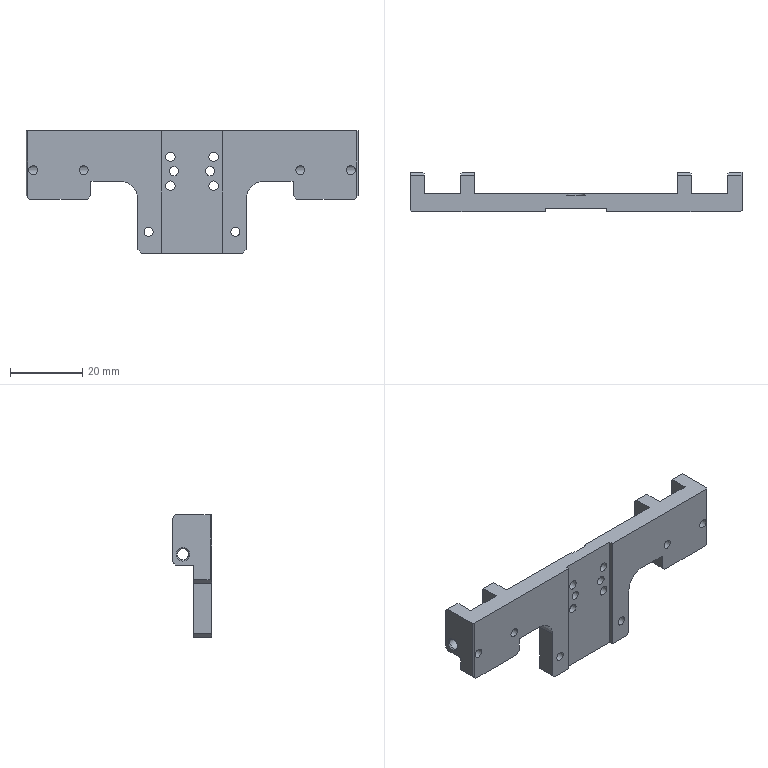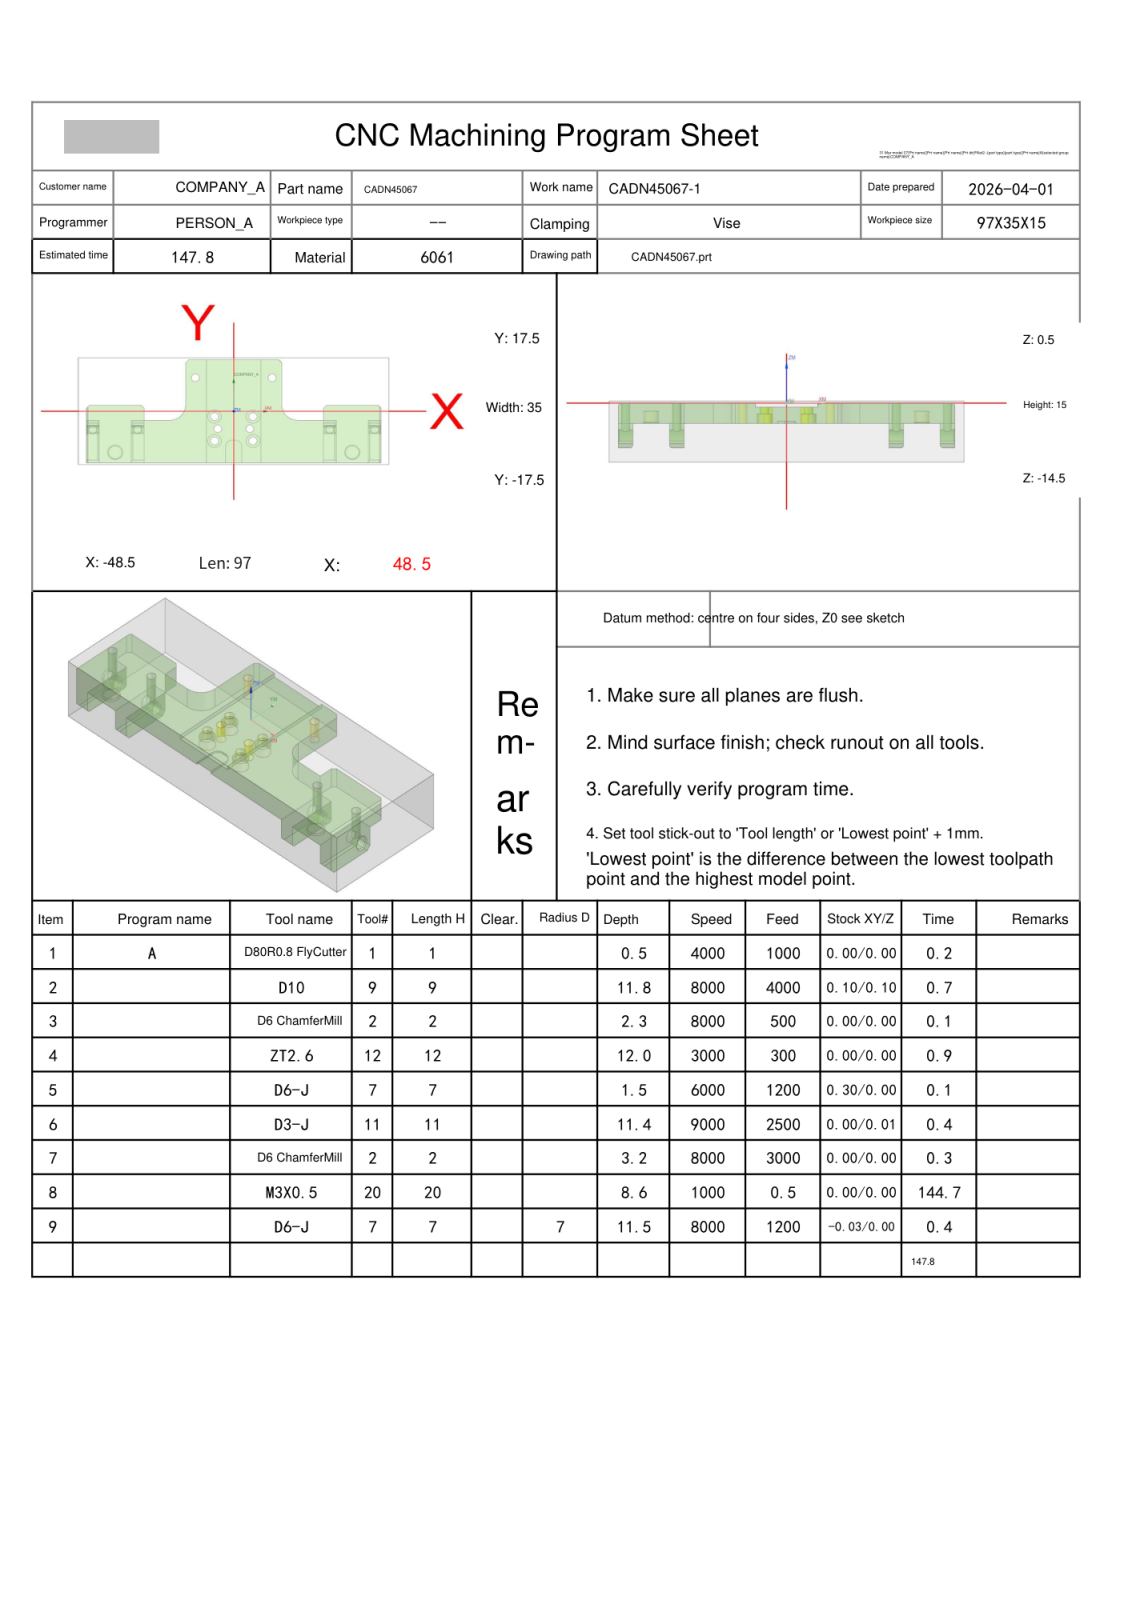NC program | NX | posted by the shop | part box 92 x 11 x 34 mm
Lines 974 to 3207 of 3207, first 1600 of 2234 lines:
N6 T11 M06
(D3-J  D=3. R=0. H=11 ce=0.00 di=0.01)
G00 G90 G54 X-26.294 Y2.051 M03 S9000
G43 H11 Z20.
M08
Z.154
G01 X-26.298 Y2.048 Z.09 F2000.
X-26.311 Y2.04 Z.031
X-26.332 Y2.027 Z-.021
X-26.357 Y2.009 Z-.068
X-26.388 Y1.987 Z-.11
X-26.421 Y1.961 Z-.147
X-26.456 Y1.932 Z-.178
X-26.491 Y1.9 Z-.206
X-26.525 Y1.865 Z-.229
X-26.556 Y1.828 Z-.248
X-26.584 Y1.79 Z-.264
X-26.607 Y1.75 Z-.276
X-26.623 Y1.708 Z-.285
X-26.631 Y1.667 Z-.291
X-26.63 Y1.625 Z-.295
X-26.618 Y1.583 Z-.296
G02 X-26.5 Y1. I-1.382 J-.583 F2500.
G01 Y-1.5
X-22.976
X-22.948 Y-1.485 Z-.297
X-22.944 Y-1.443 Z-.299
X-22.962 Y-1.377 Z-.304
X-23.001 Y-1.289 Z-.309
X-23.059 Y-1.182 Z-.316
X-23.134 Y-1.06 Z-.324
X-23.278 Y-.848 Z-.338
X-23.459 Y-.609 Z-.355
X-23.693 Y-.323 Z-.376
X-24. Y.01 Z-.403
X-24.329 Y.326 Z-.43
X-24.677 Y.621 Z-.458
X-25.039 Y.89 Z-.485
X-25.409 Y1.129 Z-.512
X-25.66 Y1.268 Z-.529
X-25.823 Y1.352 Z-.539
X-25.98 Y1.426 Z-.55
X-26.204 Y1.522 Z-.564
X-26.33 Y1.568 Z-.572
X-26.438 Y1.601 Z-.579
X-26.524 Y1.62 Z-.584
X-26.585 Y1.624 Z-.588
X-26.617 Y1.612 Z-.591
X-26.618 Y1.583 Z-.592
G02 X-26.5 Y1. I-1.382 J-.583
G01 Y-1.5
X-22.976
X-22.948 Y-1.485 Z-.593
X-22.944 Y-1.443 Z-.595
X-22.962 Y-1.377 Z-.6
X-23.001 Y-1.289 Z-.605
X-23.059 Y-1.182 Z-.612
X-23.134 Y-1.06 Z-.62
X-23.278 Y-.848 Z-.634
X-23.459 Y-.609 Z-.651
X-23.693 Y-.323 Z-.672
X-24. Y.01 Z-.699
X-24.329 Y.326 Z-.726
X-24.677 Y.621 Z-.754
X-25.039 Y.89 Z-.781
X-25.409 Y1.129 Z-.808
X-25.66 Y1.268 Z-.825
X-25.823 Y1.352 Z-.835
X-25.98 Y1.426 Z-.846
X-26.204 Y1.522 Z-.86
X-26.33 Y1.568 Z-.868
X-26.438 Y1.601 Z-.875
X-26.524 Y1.62 Z-.88
X-26.585 Y1.624 Z-.884
X-26.617 Y1.612 Z-.887
X-26.618 Y1.583 Z-.888
G02 X-26.5 Y1. I-1.382 J-.583
G01 Y-1.5
X-22.976
X-22.948 Y-1.485 Z-.889
X-22.944 Y-1.443 Z-.891
X-22.962 Y-1.377 Z-.895
X-23.001 Y-1.289 Z-.901
X-23.059 Y-1.182 Z-.908
X-23.134 Y-1.06 Z-.916
X-23.278 Y-.848 Z-.93
X-23.459 Y-.609 Z-.947
X-23.693 Y-.323 Z-.968
X-24. Y.01 Z-.995
X-24.329 Y.326 Z-1.022
X-24.677 Y.621 Z-1.05
X-25.039 Y.89 Z-1.077
X-25.409 Y1.129 Z-1.104
X-25.66 Y1.268 Z-1.121
X-25.823 Y1.352 Z-1.131
X-25.98 Y1.426 Z-1.141
X-26.204 Y1.522 Z-1.156
X-26.33 Y1.568 Z-1.164
X-26.438 Y1.601 Z-1.171
X-26.524 Y1.62 Z-1.176
X-26.585 Y1.624 Z-1.18
X-26.617 Y1.612 Z-1.183
X-26.618 Y1.583 Z-1.184
G02 X-26.5 Y1. I-1.382 J-.583
G01 Y-1.5
X-22.976
X-22.948 Y-1.485 Z-1.185
X-22.944 Y-1.443 Z-1.187
X-22.962 Y-1.377 Z-1.191
X-23.001 Y-1.289 Z-1.197
X-23.059 Y-1.182 Z-1.204
X-23.134 Y-1.06 Z-1.212
X-23.278 Y-.848 Z-1.226
X-23.459 Y-.609 Z-1.243
X-23.693 Y-.323 Z-1.264
X-24. Y.01 Z-1.29
X-24.329 Y.326 Z-1.318
X-24.677 Y.621 Z-1.346
X-25.039 Y.89 Z-1.373
X-25.409 Y1.129 Z-1.4
X-25.66 Y1.268 Z-1.417
X-25.823 Y1.352 Z-1.427
X-25.98 Y1.426 Z-1.437
X-26.204 Y1.522 Z-1.452
X-26.33 Y1.568 Z-1.46
X-26.438 Y1.601 Z-1.467
X-26.524 Y1.62 Z-1.472
X-26.585 Y1.624 Z-1.476
X-26.617 Y1.612 Z-1.479
X-26.618 Y1.583 Z-1.48
G02 X-26.5 Y1. I-1.382 J-.583
G01 Y-1.5
X-22.976
X-22.948 Y-1.485 Z-1.481
X-22.944 Y-1.443 Z-1.483
X-22.962 Y-1.377 Z-1.487
X-23.001 Y-1.289 Z-1.493
X-23.059 Y-1.182 Z-1.5
X-23.134 Y-1.06 Z-1.508
X-23.278 Y-.848 Z-1.522
X-23.459 Y-.609 Z-1.539
X-23.693 Y-.323 Z-1.56
X-24. Y.01 Z-1.586
X-24.329 Y.326 Z-1.614
X-24.677 Y.621 Z-1.642
X-25.039 Y.89 Z-1.669
X-25.409 Y1.129 Z-1.696
X-25.66 Y1.268 Z-1.712
X-25.823 Y1.352 Z-1.723
X-25.98 Y1.426 Z-1.733
X-26.204 Y1.522 Z-1.748
X-26.33 Y1.568 Z-1.756
X-26.438 Y1.601 Z-1.762
X-26.524 Y1.62 Z-1.768
X-26.585 Y1.624 Z-1.772
X-26.617 Y1.612 Z-1.775
X-26.618 Y1.583 Z-1.776
G02 X-26.5 Y1. I-1.382 J-.583
G01 Y-1.5
X-22.976
X-22.948 Y-1.485 Z-1.777
X-22.944 Y-1.443 Z-1.779
X-22.962 Y-1.377 Z-1.783
X-23.001 Y-1.289 Z-1.789
X-23.059 Y-1.182 Z-1.796
X-23.134 Y-1.06 Z-1.804
X-23.278 Y-.848 Z-1.818
X-23.459 Y-.609 Z-1.835
X-23.693 Y-.323 Z-1.856
X-24. Y.01 Z-1.882
X-24.329 Y.326 Z-1.91
X-24.677 Y.621 Z-1.938
X-25.039 Y.89 Z-1.965
X-25.409 Y1.129 Z-1.991
X-25.66 Y1.268 Z-2.008
X-25.823 Y1.352 Z-2.019
X-25.98 Y1.426 Z-2.029
X-26.204 Y1.522 Z-2.044
X-26.33 Y1.568 Z-2.052
X-26.438 Y1.601 Z-2.058
X-26.524 Y1.62 Z-2.064
X-26.585 Y1.624 Z-2.068
X-26.617 Y1.612 Z-2.071
X-26.618 Y1.583 Z-2.072
G02 X-26.5 Y1. I-1.382 J-.583
G01 Y-1.5
X-22.976
X-22.948 Y-1.485 Z-2.073
X-22.944 Y-1.443 Z-2.075
X-22.962 Y-1.377 Z-2.079
X-23.001 Y-1.289 Z-2.085
X-23.059 Y-1.182 Z-2.092
X-23.134 Y-1.06 Z-2.1
X-23.278 Y-.848 Z-2.114
X-23.459 Y-.609 Z-2.131
X-23.693 Y-.323 Z-2.152
X-24. Y.01 Z-2.178
X-24.329 Y.326 Z-2.206
X-24.677 Y.621 Z-2.233
X-25.039 Y.89 Z-2.261
X-25.409 Y1.129 Z-2.287
X-25.66 Y1.268 Z-2.304
X-25.823 Y1.352 Z-2.315
X-25.98 Y1.426 Z-2.325
X-26.204 Y1.522 Z-2.34
X-26.33 Y1.568 Z-2.348
X-26.438 Y1.601 Z-2.354
X-26.524 Y1.62 Z-2.36
X-26.585 Y1.624 Z-2.364
X-26.617 Y1.612 Z-2.367
X-26.618 Y1.583 Z-2.368
G02 X-26.5 Y1. I-1.382 J-.583
G01 Y-1.5
X-22.976
X-22.948 Y-1.485
X-22.944 Y-1.443 Z-2.371
X-22.962 Y-1.377 Z-2.375
X-23.001 Y-1.289 Z-2.381
X-23.059 Y-1.182 Z-2.388
X-23.134 Y-1.06 Z-2.396
X-23.278 Y-.848 Z-2.41
X-23.459 Y-.609 Z-2.427
X-23.693 Y-.323 Z-2.448
X-24. Y.01 Z-2.474
X-24.329 Y.326 Z-2.502
X-24.677 Y.621 Z-2.529
X-25.039 Y.89 Z-2.557
X-25.409 Y1.129 Z-2.583
X-25.66 Y1.268 Z-2.6
X-25.823 Y1.352 Z-2.611
X-25.98 Y1.426 Z-2.621
X-26.204 Y1.522 Z-2.635
X-26.33 Y1.568 Z-2.643
X-26.438 Y1.601 Z-2.65
X-26.524 Y1.62 Z-2.656
X-26.585 Y1.624 Z-2.66
X-26.617 Y1.612 Z-2.663
X-26.618 Y1.583 Z-2.664
G02 X-26.5 Y1. I-1.382 J-.583
G01 Y-1.5
X-22.976
X-22.948 Y-1.485
X-22.944 Y-1.443 Z-2.667
X-22.962 Y-1.377 Z-2.671
X-23.001 Y-1.289 Z-2.677
X-23.059 Y-1.182 Z-2.684
X-23.134 Y-1.06 Z-2.692
X-23.278 Y-.848 Z-2.706
X-23.459 Y-.609 Z-2.723
X-23.693 Y-.323 Z-2.744
X-24. Y.01 Z-2.77
X-24.329 Y.326 Z-2.798
X-24.677 Y.621 Z-2.825
X-25.039 Y.89 Z-2.853
X-25.409 Y1.129 Z-2.879
X-25.66 Y1.268 Z-2.896
X-25.823 Y1.352 Z-2.907
X-25.98 Y1.426 Z-2.917
X-26.204 Y1.522 Z-2.931
X-26.33 Y1.568 Z-2.939
X-26.438 Y1.601 Z-2.946
X-26.524 Y1.62 Z-2.952
X-26.585 Y1.624 Z-2.956
X-26.617 Y1.612 Z-2.959
X-26.618 Y1.583
G02 X-26.5 Y1. I-1.382 J-.583
G01 Y-1.5
X-22.976
X-22.948 Y-1.485 Z-2.96
X-22.944 Y-1.443 Z-2.963
X-22.962 Y-1.377 Z-2.967
X-23.001 Y-1.289 Z-2.973
X-23.059 Y-1.182 Z-2.979
X-23.134 Y-1.06 Z-2.987
X-23.278 Y-.848 Z-3.002
X-23.459 Y-.609 Z-3.019
X-23.693 Y-.323 Z-3.04
X-24. Y.01 Z-3.066
X-24.329 Y.326 Z-3.094
X-24.677 Y.621 Z-3.121
X-25.039 Y.89 Z-3.149
X-25.409 Y1.129 Z-3.175
X-25.66 Y1.268 Z-3.192
X-25.823 Y1.352 Z-3.203
X-25.98 Y1.426 Z-3.213
X-26.204 Y1.522 Z-3.227
X-26.33 Y1.568 Z-3.235
X-26.438 Y1.601 Z-3.242
X-26.524 Y1.62 Z-3.248
X-26.585 Y1.624 Z-3.252
X-26.617 Y1.612 Z-3.255
X-26.618 Y1.583
G02 X-26.5 Y1. I-1.382 J-.583
G01 Y-1.5
X-22.976
X-22.948 Y-1.485 Z-3.256
X-22.944 Y-1.443 Z-3.259
X-22.962 Y-1.377 Z-3.263
X-23.001 Y-1.289 Z-3.269
X-23.059 Y-1.182 Z-3.275
X-23.134 Y-1.06 Z-3.283
X-23.278 Y-.848 Z-3.298
X-23.459 Y-.609 Z-3.315
X-23.693 Y-.323 Z-3.336
X-24. Y.01 Z-3.362
X-24.329 Y.326 Z-3.39
X-24.677 Y.621 Z-3.417
X-25.039 Y.89 Z-3.445
X-25.409 Y1.129 Z-3.471
X-25.66 Y1.268 Z-3.488
X-25.823 Y1.352 Z-3.499
X-25.98 Y1.426 Z-3.509
X-26.204 Y1.522 Z-3.523
X-26.33 Y1.568 Z-3.531
X-26.438 Y1.601 Z-3.538
X-26.524 Y1.62 Z-3.544
X-26.585 Y1.624 Z-3.548
X-26.617 Y1.612 Z-3.55
X-26.618 Y1.583 Z-3.551
G02 X-26.5 Y1. I-1.382 J-.583
G01 Y-1.5
X-22.976
X-22.948 Y-1.485 Z-3.552
X-22.944 Y-1.443 Z-3.555
X-22.962 Y-1.377 Z-3.559
X-23.001 Y-1.289 Z-3.565
X-23.059 Y-1.182 Z-3.571
X-23.134 Y-1.06 Z-3.579
X-23.278 Y-.848 Z-3.594
X-23.459 Y-.609 Z-3.61
X-23.693 Y-.323 Z-3.632
X-24. Y.01 Z-3.658
X-24.329 Y.326 Z-3.685
X-24.677 Y.621 Z-3.713
X-25.039 Y.89 Z-3.741
X-25.409 Y1.129 Z-3.767
X-25.66 Y1.268 Z-3.784
X-25.823 Y1.352 Z-3.795
X-25.98 Y1.426 Z-3.805
X-26.204 Y1.522 Z-3.819
X-26.33 Y1.568 Z-3.827
X-26.438 Y1.601 Z-3.834
X-26.524 Y1.62 Z-3.84
X-26.585 Y1.624 Z-3.844
X-26.617 Y1.612 Z-3.846
X-26.618 Y1.583 Z-3.847
G02 X-26.5 Y1. I-1.382 J-.583
G01 Y-1.5
X-22.976
X-22.948 Y-1.485 Z-3.848
X-22.944 Y-1.443 Z-3.851
X-22.962 Y-1.377 Z-3.855
X-23.001 Y-1.289 Z-3.86
X-23.059 Y-1.182 Z-3.867
X-23.134 Y-1.06 Z-3.875
X-23.278 Y-.848 Z-3.89
X-23.459 Y-.609 Z-3.906
X-23.693 Y-.323 Z-3.927
X-24. Y.01 Z-3.954
X-24.329 Y.326 Z-3.981
X-24.677 Y.621 Z-4.009
X-25.039 Y.89 Z-4.037
X-25.409 Y1.129 Z-4.063
X-25.66 Y1.268 Z-4.08
X-25.823 Y1.352 Z-4.091
X-25.98 Y1.426 Z-4.101
X-26.204 Y1.522 Z-4.115
X-26.33 Y1.568 Z-4.123
X-26.438 Y1.601 Z-4.13
X-26.524 Y1.62 Z-4.136
X-26.585 Y1.624 Z-4.14
X-26.617 Y1.612 Z-4.142
X-26.618 Y1.583 Z-4.143
G02 X-26.5 Y1. I-1.382 J-.583
G01 Y-1.5
X-22.976
X-22.948 Y-1.485 Z-4.144
X-22.944 Y-1.443 Z-4.147
X-22.962 Y-1.377 Z-4.151
X-23.001 Y-1.289 Z-4.156
X-23.059 Y-1.182 Z-4.163
X-23.134 Y-1.06 Z-4.171
X-23.278 Y-.848 Z-4.186
X-23.459 Y-.609 Z-4.202
X-23.693 Y-.323 Z-4.223
X-24. Y.01 Z-4.25
X-24.329 Y.326 Z-4.277
X-24.677 Y.621 Z-4.305
X-25.039 Y.89 Z-4.333
X-25.409 Y1.129 Z-4.359
X-25.66 Y1.268 Z-4.376
X-25.823 Y1.352 Z-4.387
X-25.98 Y1.426 Z-4.397
X-26.204 Y1.522 Z-4.411
X-26.33 Y1.568 Z-4.419
X-26.438 Y1.601 Z-4.426
X-26.524 Y1.62 Z-4.432
X-26.585 Y1.624 Z-4.436
X-26.617 Y1.612 Z-4.438
X-26.618 Y1.583 Z-4.439
G02 X-26.5 Y1. I-1.382 J-.583
G01 Y-1.5
X-22.976
X-22.948 Y-1.485 Z-4.44
X-22.944 Y-1.443 Z-4.443
X-22.962 Y-1.377 Z-4.447
X-23.001 Y-1.289 Z-4.452
X-23.059 Y-1.182 Z-4.459
X-23.134 Y-1.06 Z-4.467
X-23.278 Y-.848 Z-4.481
X-23.459 Y-.609 Z-4.498
X-23.693 Y-.323 Z-4.519
X-24. Y.01 Z-4.546
X-24.329 Y.326 Z-4.573
X-24.677 Y.621 Z-4.601
X-25.039 Y.89 Z-4.628
X-25.409 Y1.129 Z-4.655
X-25.66 Y1.268 Z-4.672
X-25.823 Y1.352 Z-4.683
X-25.98 Y1.426 Z-4.693
X-26.204 Y1.522 Z-4.707
X-26.33 Y1.568 Z-4.715
X-26.438 Y1.601 Z-4.722
X-26.524 Y1.62 Z-4.728
X-26.585 Y1.624 Z-4.732
X-26.617 Y1.612 Z-4.734
X-26.618 Y1.583 Z-4.735
G02 X-26.5 Y1. I-1.382 J-.583
G01 Y-1.5
X-22.976
X-22.948 Y-1.485 Z-4.736
X-22.944 Y-1.443 Z-4.739
X-22.962 Y-1.377 Z-4.743
X-23.001 Y-1.289 Z-4.748
X-23.059 Y-1.182 Z-4.755
X-23.134 Y-1.06 Z-4.763
X-23.278 Y-.848 Z-4.777
X-23.459 Y-.609 Z-4.794
X-23.693 Y-.323 Z-4.815
X-24. Y.01 Z-4.842
X-24.33 Y.326 Z-4.869
X-24.677 Y.621 Z-4.897
X-25.039 Y.89 Z-4.924
X-25.41 Y1.129 Z-4.951
X-25.66 Y1.268 Z-4.968
X-25.823 Y1.352 Z-4.979
X-25.98 Y1.426 Z-4.989
X-26.204 Y1.522 Z-5.003
X-26.33 Y1.568 Z-5.011
X-26.438 Y1.601 Z-5.018
X-26.524 Y1.62 Z-5.023
X-26.585 Y1.624 Z-5.028
X-26.617 Y1.612 Z-5.03
X-26.618 Y1.583 Z-5.031
G02 X-26.5 Y1. I-1.382 J-.583
G01 Y-1.5
X-22.969
X-22.941 Y-1.485 Z-5.032
X-22.937 Y-1.443 Z-5.035
X-22.956 Y-1.377 Z-5.039
X-22.995 Y-1.289 Z-5.044
X-23.053 Y-1.182 Z-5.051
X-23.128 Y-1.06 Z-5.059
X-23.273 Y-.848 Z-5.073
X-23.454 Y-.609 Z-5.09
X-23.688 Y-.323 Z-5.111
X-23.996 Y.01 Z-5.138
X-24.326 Y.326 Z-5.165
X-24.674 Y.621 Z-5.193
X-25.036 Y.89 Z-5.22
X-25.408 Y1.129 Z-5.247
X-25.659 Y1.268 Z-5.264
X-25.822 Y1.352 Z-5.275
X-25.979 Y1.426 Z-5.285
X-26.204 Y1.522 Z-5.299
X-26.33 Y1.568 Z-5.307
X-26.438 Y1.601 Z-5.314
X-26.524 Y1.62 Z-5.319
X-26.585 Y1.624 Z-5.324
X-26.617 Y1.612 Z-5.326
X-26.618 Y1.583 Z-5.327
G02 X-26.5 Y1. I-1.382 J-.583
G01 Y-1.5
X-22.969
X-22.941 Y-1.485 Z-5.328
X-22.937 Y-1.443 Z-5.331
X-22.956 Y-1.377 Z-5.335
X-22.995 Y-1.289 Z-5.34
X-23.053 Y-1.182 Z-5.347
X-23.128 Y-1.06 Z-5.355
X-23.273 Y-.848 Z-5.369
X-23.454 Y-.609 Z-5.386
X-23.688 Y-.323 Z-5.407
X-23.996 Y.01 Z-5.434
X-24.326 Y.326 Z-5.461
X-24.674 Y.621 Z-5.489
X-25.036 Y.89 Z-5.516
X-25.408 Y1.129 Z-5.543
X-25.659 Y1.268 Z-5.56
X-25.822 Y1.352 Z-5.57
X-25.979 Y1.426 Z-5.581
X-26.204 Y1.522 Z-5.595
X-26.33 Y1.568 Z-5.603
X-26.438 Y1.601 Z-5.61
X-26.524 Y1.62 Z-5.615
X-26.585 Y1.624 Z-5.619
X-26.617 Y1.612 Z-5.622
X-26.618 Y1.583 Z-5.623
G02 X-26.5 Y1. I-1.382 J-.583
G01 Y-1.5
X-22.969
X-22.941 Y-1.485 Z-5.624
X-22.937 Y-1.443 Z-5.626
X-22.956 Y-1.377 Z-5.631
X-22.995 Y-1.289 Z-5.636
X-23.053 Y-1.182 Z-5.643
X-23.128 Y-1.06 Z-5.651
X-23.273 Y-.848 Z-5.665
X-23.454 Y-.609 Z-5.682
X-23.688 Y-.323 Z-5.703
X-23.996 Y.01 Z-5.73
X-24.326 Y.326 Z-5.757
X-24.674 Y.621 Z-5.785
X-25.036 Y.89 Z-5.812
X-25.408 Y1.129 Z-5.839
X-25.659 Y1.268 Z-5.856
X-25.822 Y1.352 Z-5.866
X-25.979 Y1.426 Z-5.877
X-26.204 Y1.522 Z-5.891
X-26.33 Y1.568 Z-5.899
X-26.438 Y1.601 Z-5.906
X-26.524 Y1.62 Z-5.911
X-26.585 Y1.624 Z-5.915
X-26.617 Y1.612 Z-5.918
X-26.618 Y1.583 Z-5.919
G02 X-26.5 Y1. I-1.382 J-.583
G01 Y-1.5
X-22.969
X-22.941 Y-1.485 Z-5.92
X-22.937 Y-1.443 Z-5.922
X-22.956 Y-1.377 Z-5.927
X-22.995 Y-1.289 Z-5.932
X-23.053 Y-1.182 Z-5.939
X-23.128 Y-1.06 Z-5.947
X-23.273 Y-.848 Z-5.961
X-23.454 Y-.609 Z-5.978
X-23.688 Y-.323 Z-5.999
X-23.996 Y.01 Z-6.026
X-24.326 Y.326 Z-6.053
X-24.674 Y.621 Z-6.081
X-25.036 Y.89 Z-6.108
X-25.408 Y1.129 Z-6.135
X-25.659 Y1.268 Z-6.152
X-25.822 Y1.352 Z-6.162
X-25.979 Y1.426 Z-6.172
X-26.204 Y1.522 Z-6.187
X-26.33 Y1.568 Z-6.195
X-26.438 Y1.601 Z-6.202
X-26.524 Y1.62 Z-6.207
X-26.585 Y1.624 Z-6.211
X-26.617 Y1.612 Z-6.214
X-26.618 Y1.583 Z-6.215
G02 X-26.5 Y1. I-1.382 J-.583
G01 Y-1.5
X-22.969
X-22.941 Y-1.485 Z-6.216
X-22.937 Y-1.443 Z-6.218
X-22.956 Y-1.377 Z-6.222
X-22.995 Y-1.289 Z-6.228
X-23.053 Y-1.182 Z-6.235
X-23.128 Y-1.06 Z-6.243
X-23.273 Y-.848 Z-6.257
X-23.454 Y-.609 Z-6.274
X-23.688 Y-.323 Z-6.295
X-23.996 Y.01 Z-6.322
X-24.326 Y.326 Z-6.349
X-24.674 Y.621 Z-6.377
X-25.036 Y.89 Z-6.404
X-25.408 Y1.129 Z-6.431
X-25.659 Y1.268 Z-6.448
X-25.822 Y1.352 Z-6.458
X-25.979 Y1.426 Z-6.468
X-26.204 Y1.522 Z-6.483
X-26.33 Y1.568 Z-6.491
X-26.438 Y1.601 Z-6.498
X-26.524 Y1.62 Z-6.503
X-26.585 Y1.624 Z-6.507
X-26.617 Y1.612 Z-6.51
X-26.618 Y1.583 Z-6.511
G02 X-26.5 Y1. I-1.382 J-.583
G01 Y-1.5
X-22.969
X-22.941 Y-1.485 Z-6.512
X-22.937 Y-1.443 Z-6.514
X-22.956 Y-1.377 Z-6.518
X-22.995 Y-1.289 Z-6.524
X-23.053 Y-1.182 Z-6.531
X-23.128 Y-1.06 Z-6.539
X-23.273 Y-.848 Z-6.553
X-23.454 Y-.609 Z-6.57
X-23.688 Y-.323 Z-6.591
X-23.996 Y.01 Z-6.617
X-24.326 Y.326 Z-6.645
X-24.674 Y.621 Z-6.673
X-25.036 Y.89 Z-6.7
X-25.408 Y1.129 Z-6.727
X-25.659 Y1.268 Z-6.744
X-25.822 Y1.352 Z-6.754
X-25.979 Y1.426 Z-6.764
X-26.204 Y1.522 Z-6.779
X-26.33 Y1.568 Z-6.787
X-26.438 Y1.601 Z-6.794
X-26.524 Y1.62 Z-6.799
X-26.585 Y1.624 Z-6.803
X-26.617 Y1.612 Z-6.806
X-26.618 Y1.583 Z-6.807
G02 X-26.5 Y1. I-1.382 J-.583
G01 Y-1.5
X-22.969
X-22.941 Y-1.485 Z-6.808
X-22.937 Y-1.443 Z-6.81
X-22.956 Y-1.377 Z-6.814
X-22.995 Y-1.289 Z-6.82
X-23.053 Y-1.182 Z-6.827
X-23.128 Y-1.06 Z-6.835
X-23.273 Y-.848 Z-6.849
X-23.454 Y-.609 Z-6.866
X-23.688 Y-.323 Z-6.887
X-23.996 Y.01 Z-6.913
X-24.326 Y.326 Z-6.941
X-24.674 Y.621 Z-6.969
X-25.036 Y.89 Z-6.996
X-25.408 Y1.129 Z-7.022
X-25.659 Y1.268 Z-7.039
X-25.822 Y1.352 Z-7.05
X-25.979 Y1.426 Z-7.06
X-26.204 Y1.522 Z-7.075
X-26.33 Y1.568 Z-7.083
X-26.438 Y1.601 Z-7.089
X-26.524 Y1.62 Z-7.095
X-26.585 Y1.624 Z-7.099
X-26.617 Y1.612 Z-7.102
X-26.618 Y1.583 Z-7.103
G02 X-26.5 Y1. I-1.382 J-.583
G01 Y-1.5
X-22.969
X-22.941 Y-1.485 Z-7.104
X-22.937 Y-1.443 Z-7.106
X-22.956 Y-1.377 Z-7.11
X-22.995 Y-1.289 Z-7.116
X-23.053 Y-1.182 Z-7.123
X-23.128 Y-1.06 Z-7.131
X-23.273 Y-.848 Z-7.145
X-23.454 Y-.609 Z-7.162
X-23.688 Y-.323 Z-7.183
X-23.996 Y.01 Z-7.209
X-24.326 Y.326 Z-7.237
X-24.674 Y.621 Z-7.264
X-25.036 Y.89 Z-7.292
X-25.408 Y1.129 Z-7.318
X-25.659 Y1.268 Z-7.335
X-25.822 Y1.352 Z-7.346
X-25.979 Y1.426 Z-7.356
X-26.204 Y1.522 Z-7.371
X-26.33 Y1.568 Z-7.379
X-26.438 Y1.601 Z-7.385
X-26.524 Y1.62 Z-7.391
X-26.585 Y1.624 Z-7.395
X-26.617 Y1.612 Z-7.398
X-26.618 Y1.583 Z-7.399
G02 X-26.5 Y1. I-1.382 J-.583
G01 Y-1.5
X-22.969
X-22.941 Y-1.485 Z-7.4
X-22.937 Y-1.443 Z-7.402
X-22.956 Y-1.377 Z-7.406
X-22.995 Y-1.289 Z-7.412
X-23.053 Y-1.182 Z-7.419
X-23.128 Y-1.06 Z-7.427
X-23.273 Y-.848 Z-7.441
X-23.454 Y-.609 Z-7.458
X-23.688 Y-.323 Z-7.479
X-23.996 Y.01 Z-7.505
X-24.326 Y.326 Z-7.533
X-24.674 Y.621 Z-7.56
X-25.036 Y.89 Z-7.588
X-25.408 Y1.129 Z-7.614
X-25.659 Y1.268 Z-7.631
X-25.822 Y1.352 Z-7.642
X-25.979 Y1.426 Z-7.652
X-26.204 Y1.522 Z-7.667
X-26.33 Y1.568 Z-7.675
X-26.438 Y1.601 Z-7.681
X-26.524 Y1.62 Z-7.687
X-26.585 Y1.624 Z-7.691
X-26.617 Y1.612 Z-7.694
X-26.618 Y1.583 Z-7.695
G02 X-26.5 Y1. I-1.382 J-.583
G01 Y-1.5
X-22.969
X-22.941 Y-1.485
X-22.937 Y-1.443 Z-7.698
X-22.956 Y-1.377 Z-7.702
X-22.995 Y-1.289 Z-7.708
X-23.053 Y-1.182 Z-7.715
X-23.128 Y-1.06 Z-7.723
X-23.273 Y-.848 Z-7.737
X-23.454 Y-.609 Z-7.754
X-23.688 Y-.323 Z-7.775
X-23.996 Y.01 Z-7.801
X-24.326 Y.326 Z-7.829
X-24.674 Y.621 Z-7.856
X-25.036 Y.89 Z-7.884
X-25.408 Y1.129 Z-7.91
X-25.659 Y1.268 Z-7.927
X-25.822 Y1.352 Z-7.938
X-25.979 Y1.426 Z-7.948
X-26.204 Y1.522 Z-7.962
X-26.33 Y1.568 Z-7.97
X-26.438 Y1.601 Z-7.977
X-26.524 Y1.62 Z-7.983
X-26.585 Y1.624 Z-7.987
X-26.617 Y1.612 Z-7.99
X-26.618 Y1.583 Z-7.991
G02 X-26.5 Y1. I-1.382 J-.583
G01 Y-1.5
X-22.969
X-22.941 Y-1.485
X-22.937 Y-1.443 Z-7.994
X-22.956 Y-1.377 Z-7.998
X-22.995 Y-1.289 Z-8.004
X-23.053 Y-1.182 Z-8.011
X-23.128 Y-1.06 Z-8.019
X-23.273 Y-.848 Z-8.033
X-23.454 Y-.609 Z-8.05
X-23.688 Y-.323 Z-8.071
X-23.996 Y.01 Z-8.097
X-24.326 Y.326 Z-8.125
X-24.674 Y.621 Z-8.152
X-25.036 Y.89 Z-8.18
X-25.408 Y1.129 Z-8.206
X-25.659 Y1.268 Z-8.223
X-25.822 Y1.352 Z-8.234
X-25.979 Y1.426 Z-8.244
X-26.204 Y1.522 Z-8.258
X-26.33 Y1.568 Z-8.266
X-26.438 Y1.601 Z-8.273
X-26.524 Y1.62 Z-8.279
X-26.585 Y1.624 Z-8.283
X-26.617 Y1.612 Z-8.286
X-26.618 Y1.583
G02 X-26.5 Y1. I-1.382 J-.583
G01 Y-1.5
X-22.969
X-22.941 Y-1.485 Z-8.287
X-22.937 Y-1.443 Z-8.29
X-22.956 Y-1.377 Z-8.294
X-22.995 Y-1.289 Z-8.3
X-23.053 Y-1.182 Z-8.307
X-23.128 Y-1.06 Z-8.314
X-23.273 Y-.848 Z-8.329
X-23.454 Y-.609 Z-8.346
X-23.688 Y-.323 Z-8.367
X-23.996 Y.01 Z-8.393
X-24.326 Y.326 Z-8.421
X-24.674 Y.621 Z-8.448
X-25.036 Y.89 Z-8.476
X-25.408 Y1.129 Z-8.502
X-25.659 Y1.268 Z-8.519
X-25.822 Y1.352 Z-8.53
X-25.979 Y1.426 Z-8.54
X-26.204 Y1.522 Z-8.554
X-26.33 Y1.568 Z-8.562
X-26.438 Y1.601 Z-8.569
X-26.524 Y1.62 Z-8.575
X-26.585 Y1.624 Z-8.579
X-26.617 Y1.612 Z-8.582
X-26.618 Y1.583
G02 X-26.5 Y1. I-1.382 J-.583
G01 Y-1.5
X-22.969
X-22.941 Y-1.485 Z-8.583
X-22.937 Y-1.443 Z-8.586
X-22.956 Y-1.377 Z-8.59
X-22.995 Y-1.289 Z-8.596
X-23.053 Y-1.182 Z-8.602
X-23.128 Y-1.06 Z-8.61
X-23.273 Y-.848 Z-8.625
X-23.454 Y-.609 Z-8.642
X-23.688 Y-.323 Z-8.663
X-23.996 Y.01 Z-8.689
X-24.326 Y.326 Z-8.716
X-24.674 Y.621 Z-8.744
X-25.036 Y.89 Z-8.772
X-25.408 Y1.129 Z-8.798
X-25.659 Y1.269 Z-8.815
X-25.822 Y1.352 Z-8.826
X-25.979 Y1.426 Z-8.836
X-26.204 Y1.522 Z-8.85
X-26.33 Y1.568 Z-8.858
X-26.438 Y1.601 Z-8.865
X-26.524 Y1.62 Z-8.871
X-26.585 Y1.624 Z-8.875
X-26.617 Y1.612 Z-8.877
X-26.618 Y1.583 Z-8.878
G02 X-26.5 Y1. I-1.382 J-.583
G01 Y-1.5
X-22.969
X-22.941 Y-1.485 Z-8.879
X-22.937 Y-1.443 Z-8.882
X-22.956 Y-1.377 Z-8.886
X-22.995 Y-1.289 Z-8.892
X-23.053 Y-1.182 Z-8.898
X-23.128 Y-1.06 Z-8.906
X-23.273 Y-.848 Z-8.921
X-23.454 Y-.609 Z-8.937
X-23.688 Y-.323 Z-8.958
X-23.996 Y.01 Z-8.985
X-24.326 Y.326 Z-9.012
X-24.674 Y.621 Z-9.04
X-25.036 Y.89 Z-9.068
X-25.408 Y1.129 Z-9.094
X-25.659 Y1.269 Z-9.111
X-25.822 Y1.352 Z-9.122
X-25.979 Y1.426 Z-9.132
X-26.204 Y1.522 Z-9.146
X-26.33 Y1.568 Z-9.154
X-26.438 Y1.601 Z-9.161
X-26.524 Y1.62 Z-9.167
X-26.585 Y1.624 Z-9.171
X-26.617 Y1.612 Z-9.173
X-26.618 Y1.583 Z-9.174
G02 X-26.5 Y1. I-1.382 J-.583
G01 Y-1.5
X-22.969
X-22.941 Y-1.485 Z-9.175
X-22.937 Y-1.443 Z-9.178
X-22.956 Y-1.377 Z-9.182
X-22.995 Y-1.289 Z-9.188
X-23.053 Y-1.182 Z-9.194
X-23.128 Y-1.06 Z-9.202
X-23.273 Y-.848 Z-9.217
X-23.454 Y-.609 Z-9.233
X-23.688 Y-.323 Z-9.254
X-23.996 Y.01 Z-9.281
X-24.326 Y.326 Z-9.308
X-24.674 Y.621 Z-9.336
X-25.036 Y.89 Z-9.364
X-25.408 Y1.129 Z-9.39
X-25.659 Y1.269 Z-9.407
X-25.822 Y1.352 Z-9.418
X-25.979 Y1.426 Z-9.428
X-26.204 Y1.522 Z-9.442
X-26.33 Y1.568 Z-9.45
X-26.438 Y1.601 Z-9.457
X-26.524 Y1.62 Z-9.463
X-26.585 Y1.624 Z-9.467
X-26.617 Y1.612 Z-9.469
X-26.618 Y1.583 Z-9.47
G02 X-26.5 Y1. I-1.382 J-.583
G01 Y-1.5
X-22.969
X-22.941 Y-1.485 Z-9.471
X-22.937 Y-1.443 Z-9.474
X-22.956 Y-1.377 Z-9.478
X-22.995 Y-1.289 Z-9.483
X-23.053 Y-1.182 Z-9.49
X-23.128 Y-1.06 Z-9.498
X-23.273 Y-.848 Z-9.513
X-23.454 Y-.609 Z-9.529
X-23.688 Y-.323 Z-9.55
X-23.996 Y.01 Z-9.577
X-24.326 Y.326 Z-9.604
X-24.674 Y.621 Z-9.632
X-25.036 Y.89 Z-9.659
X-25.408 Y1.129 Z-9.686
X-25.659 Y1.269 Z-9.703
X-25.822 Y1.352 Z-9.714
X-25.979 Y1.426 Z-9.724
X-26.204 Y1.522 Z-9.738
X-26.33 Y1.568 Z-9.746
X-26.438 Y1.601 Z-9.753
X-26.524 Y1.62 Z-9.759
X-26.585 Y1.624 Z-9.763
X-26.617 Y1.612 Z-9.765
X-26.618 Y1.583 Z-9.766
G02 X-26.5 Y1. I-1.382 J-.583
G01 Y-1.5
X-22.969
X-22.941 Y-1.485 Z-9.767
X-22.937 Y-1.443 Z-9.77
X-22.956 Y-1.377 Z-9.774
X-22.995 Y-1.289 Z-9.779
X-23.053 Y-1.182 Z-9.786
X-23.128 Y-1.06 Z-9.794
X-23.273 Y-.848 Z-9.809
X-23.454 Y-.609 Z-9.825
X-23.688 Y-.323 Z-9.846
X-23.996 Y.01 Z-9.873
X-24.326 Y.326 Z-9.9
X-24.674 Y.621 Z-9.928
X-25.036 Y.89 Z-9.955
X-25.408 Y1.129 Z-9.982
X-25.659 Y1.269 Z-9.999
X-25.822 Y1.352 Z-10.01
X-25.979 Y1.426 Z-10.02
X-26.204 Y1.522 Z-10.034
X-26.33 Y1.568 Z-10.042
X-26.438 Y1.601 Z-10.049
X-26.524 Y1.62 Z-10.055
X-26.585 Y1.624 Z-10.059
X-26.617 Y1.612 Z-10.061
X-26.618 Y1.583 Z-10.062
G02 X-26.5 Y1. I-1.382 J-.583
G01 Y-1.5
X-22.969
X-22.941 Y-1.485 Z-10.063
X-22.937 Y-1.443 Z-10.066
X-22.956 Y-1.377 Z-10.07
X-22.995 Y-1.289 Z-10.075
X-23.053 Y-1.182 Z-10.082
X-23.128 Y-1.06 Z-10.09
X-23.273 Y-.848 Z-10.104
X-23.454 Y-.609 Z-10.121
X-23.688 Y-.323 Z-10.142
X-23.996 Y.01 Z-10.169
X-24.326 Y.326 Z-10.196
X-24.674 Y.621 Z-10.224
X-25.036 Y.89 Z-10.251
X-25.408 Y1.129 Z-10.278
X-25.659 Y1.269 Z-10.295
X-25.822 Y1.352 Z-10.306
X-25.979 Y1.426 Z-10.316
X-26.204 Y1.522 Z-10.33
X-26.33 Y1.568 Z-10.338
X-26.438 Y1.601 Z-10.345
X-26.524 Y1.62 Z-10.35
X-26.585 Y1.624 Z-10.355
X-26.617 Y1.612 Z-10.357
X-26.618 Y1.583 Z-10.358
G02 X-26.5 Y1. I-1.382 J-.583
G01 Y-1.5
X-22.969
X-22.941 Y-1.485 Z-10.359
X-22.937 Y-1.443 Z-10.362
X-22.956 Y-1.377 Z-10.366
X-22.995 Y-1.289 Z-10.371
X-23.053 Y-1.182 Z-10.378
X-23.128 Y-1.06 Z-10.386
X-23.273 Y-.848 Z-10.4
X-23.454 Y-.609 Z-10.417
X-23.688 Y-.323 Z-10.438
X-23.996 Y.01 Z-10.465
X-24.326 Y.326 Z-10.492
X-24.674 Y.621 Z-10.52
X-25.036 Y.89 Z-10.547
X-25.408 Y1.129 Z-10.574
X-25.659 Y1.269 Z-10.591
X-25.822 Y1.352 Z-10.602
X-25.979 Y1.426 Z-10.612
X-26.204 Y1.522 Z-10.626
X-26.33 Y1.568 Z-10.634
X-26.438 Y1.601 Z-10.641
X-26.524 Y1.62 Z-10.646
X-26.585 Y1.624 Z-10.651
X-26.617 Y1.612 Z-10.653
X-26.618 Y1.583 Z-10.654
G02 X-26.5 Y1. I-1.382 J-.583
G01 Y-1.5
X-22.969
X-22.941 Y-1.485 Z-10.655
X-22.937 Y-1.443 Z-10.658
X-22.956 Y-1.377 Z-10.662
X-22.995 Y-1.289 Z-10.667
X-23.053 Y-1.182 Z-10.674
X-23.128 Y-1.06 Z-10.682
X-23.273 Y-.848 Z-10.696
X-23.454 Y-.609 Z-10.713
X-23.688 Y-.323 Z-10.734
X-23.996 Y.01 Z-10.761
X-24.326 Y.326 Z-10.788
X-24.674 Y.621 Z-10.816
X-25.036 Y.89 Z-10.843
X-25.408 Y1.129 Z-10.87
X-25.659 Y1.269 Z-10.887
X-25.822 Y1.352 Z-10.898
X-25.979 Y1.426 Z-10.908
X-26.204 Y1.522 Z-10.922
X-26.33 Y1.568 Z-10.93
X-26.438 Y1.601 Z-10.937
X-26.524 Y1.62 Z-10.942
X-26.585 Y1.624 Z-10.947
X-26.617 Y1.612 Z-10.949
X-26.618 Y1.583 Z-10.95
G02 X-26.5 Y1. I-1.382 J-.583
G01 Y-1.5
X-22.969
X-22.928 Y-1.475 Z-10.949
X-22.891 Y-1.441 Z-10.945
X-22.858 Y-1.401 Z-10.938
X-22.828 Y-1.355 Z-10.927
X-22.802 Y-1.305 Z-10.913
X-22.78 Y-1.253 Z-10.895
X-22.76 Y-1.2 Z-10.873
X-22.744 Y-1.147 Z-10.846
X-22.731 Y-1.097 Z-10.814
X-22.72 Y-1.05 Z-10.777
X-22.711 Y-1.009 Z-10.734
X-22.705 Y-.973 Z-10.685
X-22.701 Y-.947 Z-10.63
X-22.698 Y-.929 Z-10.568
X-22.697 Y-.923 Z-10.5
G00 Z20.
X22.725 Y-.914
Z.154
G01 X22.726 Y-.92 Z.086 F2000.
X22.727 Y-.938 Z.024
X22.73 Y-.965 Z-.031
X22.735 Y-1.001 Z-.08
X22.742 Y-1.043 Z-.123
X22.751 Y-1.091 Z-.16
X22.762 Y-1.142 Z-.192
X22.776 Y-1.196 Z-.219
X22.794 Y-1.25 Z-.241
X22.814 Y-1.303 Z-.259
X22.838 Y-1.354 Z-.273
X22.866 Y-1.4 Z-.284
X22.898 Y-1.441 Z-.291
X22.935 Y-1.475 Z-.295
X22.976 Y-1.5 Z-.296
X26.5 F2500.
Y1.
G02 X26.618 Y1.583 I1.5 J0.0
G01 X26.617 Y1.612 Z-.297
X26.586 Y1.624 Z-.299
X26.526 Y1.619 Z-.304
X26.442 Y1.6 Z-.309
X26.336 Y1.566 Z-.316
X26.212 Y1.519 Z-.324
X25.991 Y1.422 Z-.338
X25.736 Y1.295 Z-.355
X25.428 Y1.123 Z-.376
X25.06 Y.885 Z-.403
X24.7 Y.617 Z-.43
X24.352 Y.323 Z-.458
X24.02 Y.008 Z-.485
X23.711 Y-.323 Z-.512
X23.473 Y-.608 Z-.533
X23.336 Y-.786 Z-.545
X23.141 Y-1.06 Z-.564
X23.065 Y-1.182 Z-.572
X23.005 Y-1.288 Z-.579
X22.964 Y-1.376 Z-.584
X22.945 Y-1.443 Z-.588
X22.948 Y-1.485 Z-.591
X22.976 Y-1.5 Z-.592
X26.5
Y1.
G02 X26.618 Y1.583 I1.5 J0.0
G01 X26.617 Y1.612 Z-.593
X26.586 Y1.624 Z-.595
X26.526 Y1.619 Z-.6
X26.442 Y1.6 Z-.605
X26.336 Y1.566 Z-.612
X26.212 Y1.519 Z-.62
X25.991 Y1.422 Z-.634
X25.736 Y1.295 Z-.651
X25.428 Y1.123 Z-.672
X25.06 Y.885 Z-.699
X24.7 Y.617 Z-.726
X24.352 Y.323 Z-.754
X24.02 Y.008 Z-.781
X23.711 Y-.323 Z-.808
X23.473 Y-.608 Z-.829
X23.336 Y-.786 Z-.841
X23.141 Y-1.06 Z-.86
X23.065 Y-1.182 Z-.868
X23.005 Y-1.288 Z-.875
X22.964 Y-1.376 Z-.88
X22.945 Y-1.443 Z-.884
X22.948 Y-1.485 Z-.887
X22.976 Y-1.5 Z-.888
X26.5
Y1.
G02 X26.618 Y1.583 I1.5 J0.0
G01 X26.617 Y1.612 Z-.889
X26.586 Y1.624 Z-.891
X26.526 Y1.619 Z-.895
X26.442 Y1.6 Z-.901
X26.336 Y1.566 Z-.908
X26.212 Y1.519 Z-.916
X25.991 Y1.422 Z-.93
X25.736 Y1.295 Z-.947
X25.428 Y1.123 Z-.968
X25.06 Y.885 Z-.995
X24.7 Y.617 Z-1.022
X24.352 Y.323 Z-1.05
X24.02 Y.008 Z-1.077
X23.711 Y-.323 Z-1.104
X23.473 Y-.608 Z-1.125
X23.336 Y-.786 Z-1.137
X23.141 Y-1.06 Z-1.156
X23.065 Y-1.182 Z-1.164
X23.005 Y-1.288 Z-1.171
X22.964 Y-1.376 Z-1.176
X22.945 Y-1.443 Z-1.18
X22.948 Y-1.485 Z-1.183
X22.976 Y-1.5 Z-1.184
X26.5
Y1.
G02 X26.618 Y1.583 I1.5 J0.0
G01 X26.617 Y1.612 Z-1.185
X26.586 Y1.624 Z-1.187
X26.526 Y1.619 Z-1.191
X26.442 Y1.6 Z-1.197
X26.336 Y1.566 Z-1.204
X26.212 Y1.519 Z-1.212
X25.991 Y1.422 Z-1.226
X25.736 Y1.295 Z-1.243
X25.428 Y1.123 Z-1.264
X25.06 Y.885 Z-1.29
X24.7 Y.617 Z-1.318
X24.352 Y.323 Z-1.346
X24.02 Y.008 Z-1.373
X23.711 Y-.323 Z-1.4
X23.473 Y-.608 Z-1.421
X23.336 Y-.786 Z-1.433
X23.141 Y-1.06 Z-1.452
X23.065 Y-1.182 Z-1.46
X23.005 Y-1.288 Z-1.467
X22.964 Y-1.376 Z-1.472
X22.945 Y-1.443 Z-1.476
X22.948 Y-1.485 Z-1.479
X22.976 Y-1.5 Z-1.48
X26.5
Y1.
G02 X26.618 Y1.583 I1.5 J0.0
G01 X26.617 Y1.612 Z-1.481
X26.586 Y1.624 Z-1.483
X26.526 Y1.619 Z-1.487
X26.442 Y1.6 Z-1.493
X26.336 Y1.566 Z-1.5
X26.212 Y1.519 Z-1.508
X25.991 Y1.422 Z-1.522
X25.736 Y1.295 Z-1.539
X25.428 Y1.123 Z-1.56
X25.06 Y.885 Z-1.586
X24.7 Y.617 Z-1.614
X24.352 Y.323 Z-1.642
X24.02 Y.008 Z-1.669
X23.711 Y-.323 Z-1.696
X23.473 Y-.608 Z-1.717
X23.336 Y-.786 Z-1.729
X23.141 Y-1.06 Z-1.748
X23.065 Y-1.182 Z-1.756
X23.005 Y-1.288 Z-1.762
X22.964 Y-1.376 Z-1.768
X22.945 Y-1.443 Z-1.772
X22.948 Y-1.485 Z-1.775
X22.976 Y-1.5 Z-1.776
X26.5
Y1.
G02 X26.618 Y1.583 I1.5 J0.0
G01 X26.617 Y1.612 Z-1.777
X26.586 Y1.624 Z-1.779
X26.526 Y1.619 Z-1.783
X26.442 Y1.6 Z-1.789
X26.336 Y1.566 Z-1.796
X26.212 Y1.519 Z-1.804
X25.991 Y1.422 Z-1.818
X25.736 Y1.295 Z-1.835
X25.428 Y1.123 Z-1.856
X25.06 Y.885 Z-1.882
X24.7 Y.617 Z-1.91
X24.352 Y.323 Z-1.938
X24.02 Y.008 Z-1.965
X23.711 Y-.323 Z-1.991
X23.473 Y-.608 Z-2.013
X23.336 Y-.786 Z-2.025
X23.141 Y-1.06 Z-2.044
X23.065 Y-1.182 Z-2.052
X23.005 Y-1.288 Z-2.058
X22.964 Y-1.376 Z-2.064
X22.945 Y-1.443 Z-2.068
X22.948 Y-1.485 Z-2.071
X22.976 Y-1.5 Z-2.072
X26.5
Y1.
G02 X26.618 Y1.583 I1.5 J0.0
G01 X26.617 Y1.612 Z-2.073
X26.586 Y1.624 Z-2.075
X26.526 Y1.619 Z-2.079
X26.442 Y1.6 Z-2.085
X26.336 Y1.566 Z-2.092
X26.212 Y1.519 Z-2.1
X25.991 Y1.422 Z-2.114
X25.736 Y1.295 Z-2.131
X25.428 Y1.123 Z-2.152
X25.06 Y.885 Z-2.178
X24.7 Y.617 Z-2.206
X24.352 Y.323 Z-2.233
X24.02 Y.008 Z-2.261
X23.711 Y-.323 Z-2.287
X23.473 Y-.608 Z-2.308
X23.336 Y-.786 Z-2.321
X23.141 Y-1.06 Z-2.34
X23.065 Y-1.182 Z-2.348
X23.005 Y-1.288 Z-2.354
X22.964 Y-1.376 Z-2.36
X22.945 Y-1.443 Z-2.364
X22.948 Y-1.485 Z-2.367
X22.976 Y-1.5 Z-2.368
X26.5
Y1.
G02 X26.618 Y1.583 I1.5 J0.0
G01 X26.617 Y1.612
X26.586 Y1.624 Z-2.371
X26.526 Y1.619 Z-2.375
X26.442 Y1.6 Z-2.381
X26.336 Y1.566 Z-2.388
X26.212 Y1.519 Z-2.396
X25.991 Y1.422 Z-2.41
X25.736 Y1.295 Z-2.427
X25.428 Y1.123 Z-2.448
X25.06 Y.885 Z-2.474
X24.7 Y.617 Z-2.502
X24.352 Y.323 Z-2.529
X24.02 Y.008 Z-2.557
X23.711 Y-.323 Z-2.583
X23.473 Y-.608 Z-2.604
X23.336 Y-.786 Z-2.617
X23.141 Y-1.06 Z-2.635
X23.065 Y-1.182 Z-2.643
X23.005 Y-1.288 Z-2.65
X22.964 Y-1.376 Z-2.656
X22.945 Y-1.443 Z-2.66
X22.948 Y-1.485 Z-2.663
X22.976 Y-1.5 Z-2.664
X26.5
Y1.
G02 X26.618 Y1.583 I1.5 J0.0
G01 X26.617 Y1.612
X26.586 Y1.624 Z-2.667
X26.526 Y1.619 Z-2.671
X26.442 Y1.6 Z-2.677
X26.336 Y1.566 Z-2.684
X26.212 Y1.519 Z-2.692
X25.991 Y1.422 Z-2.706
X25.736 Y1.295 Z-2.723
X25.428 Y1.123 Z-2.744
X25.06 Y.885 Z-2.77
X24.7 Y.617 Z-2.798
X24.352 Y.323 Z-2.825
X24.02 Y.008 Z-2.853
X23.711 Y-.323 Z-2.879
X23.473 Y-.608 Z-2.9
X23.336 Y-.786 Z-2.913
X23.141 Y-1.06 Z-2.931
X23.065 Y-1.182 Z-2.939
X23.005 Y-1.288 Z-2.946
X22.964 Y-1.376 Z-2.952
X22.945 Y-1.443 Z-2.956
X22.948 Y-1.485 Z-2.959
X22.976 Y-1.5
X26.5
Y1.
G02 X26.618 Y1.583 I1.5 J0.0
G01 X26.617 Y1.612 Z-2.96
X26.586 Y1.624 Z-2.963
X26.526 Y1.619 Z-2.967
X26.442 Y1.6 Z-2.973
X26.336 Y1.566 Z-2.979
X26.212 Y1.519 Z-2.987
X25.991 Y1.422 Z-3.002
X25.736 Y1.295 Z-3.019
X25.428 Y1.123 Z-3.04
X25.06 Y.885 Z-3.066
X24.7 Y.617 Z-3.094
X24.352 Y.323 Z-3.121
X24.02 Y.008 Z-3.149
X23.711 Y-.323 Z-3.175
X23.473 Y-.608 Z-3.196
X23.336 Y-.786 Z-3.209
X23.141 Y-1.06 Z-3.227
X23.065 Y-1.182 Z-3.235
X23.005 Y-1.288 Z-3.242
X22.964 Y-1.376 Z-3.248
X22.945 Y-1.443 Z-3.252
X22.948 Y-1.485 Z-3.255
X22.976 Y-1.5
X26.5
Y1.
G02 X26.618 Y1.583 I1.5 J0.0
G01 X26.617 Y1.612 Z-3.256
X26.586 Y1.624 Z-3.259
X26.526 Y1.619 Z-3.263
X26.442 Y1.6 Z-3.269
X26.336 Y1.566 Z-3.275
X26.212 Y1.519 Z-3.283
X25.991 Y1.422 Z-3.298
X25.736 Y1.295 Z-3.315
X25.428 Y1.123 Z-3.336
X25.06 Y.885 Z-3.362
X24.7 Y.617 Z-3.39
X24.352 Y.323 Z-3.417
X24.02 Y.008 Z-3.445
X23.711 Y-.323 Z-3.471
X23.473 Y-.608 Z-3.492
X23.336 Y-.786 Z-3.505
X23.141 Y-1.06 Z-3.523
X23.065 Y-1.182 Z-3.531
X23.005 Y-1.288 Z-3.538
X22.964 Y-1.376 Z-3.544
X22.945 Y-1.443 Z-3.548
X22.948 Y-1.485 Z-3.55
X22.976 Y-1.5 Z-3.551
X26.5
Y1.
G02 X26.618 Y1.583 I1.5 J0.0
G01 X26.617 Y1.612 Z-3.552
X26.586 Y1.624 Z-3.555
X26.526 Y1.619 Z-3.559
X26.442 Y1.6 Z-3.565
X26.336 Y1.566 Z-3.571
X26.212 Y1.519 Z-3.579
X25.991 Y1.422 Z-3.594
X25.736 Y1.295 Z-3.611
X25.428 Y1.123 Z-3.632
X25.06 Y.885 Z-3.658
X24.7 Y.617 Z-3.685
X24.352 Y.323 Z-3.713
X24.02 Y.008 Z-3.741
X23.711 Y-.323 Z-3.767
X23.473 Y-.608 Z-3.788
X23.336 Y-.786 Z-3.801
X23.141 Y-1.06 Z-3.819
X23.065 Y-1.182 Z-3.827
X23.005 Y-1.288 Z-3.834
X22.964 Y-1.376 Z-3.84
X22.945 Y-1.443 Z-3.844
X22.948 Y-1.485 Z-3.846
X22.976 Y-1.5 Z-3.847
X26.5
Y1.
G02 X26.618 Y1.583 I1.5 J0.0
G01 X26.617 Y1.612 Z-3.848
X26.586 Y1.624 Z-3.851
X26.526 Y1.619 Z-3.855
X26.442 Y1.6 Z-3.86
X26.336 Y1.566 Z-3.867
X26.212 Y1.519 Z-3.875
X25.991 Y1.422 Z-3.89
X25.736 Y1.295 Z-3.906
X25.428 Y1.123 Z-3.927
X25.06 Y.885 Z-3.954
X24.7 Y.617 Z-3.981
X24.352 Y.323 Z-4.009
X24.02 Y.008 Z-4.037
X23.711 Y-.323 Z-4.063
X23.473 Y-.608 Z-4.084
X23.336 Y-.786 Z-4.097
X23.141 Y-1.06 Z-4.115
X23.065 Y-1.182 Z-4.123
X23.005 Y-1.288 Z-4.13
X22.964 Y-1.376 Z-4.136
X22.945 Y-1.443 Z-4.14
X22.948 Y-1.485 Z-4.142
X22.976 Y-1.5 Z-4.143
X26.5
Y1.
G02 X26.618 Y1.583 I1.5 J0.0
G01 X26.617 Y1.612 Z-4.144
X26.586 Y1.624 Z-4.147
X26.526 Y1.619 Z-4.151
X26.442 Y1.6 Z-4.156
X26.336 Y1.566 Z-4.163
X26.212 Y1.519 Z-4.171
X25.991 Y1.422 Z-4.186
X25.736 Y1.295 Z-4.202
X25.428 Y1.123 Z-4.223
X25.06 Y.885 Z-4.25
X24.7 Y.617 Z-4.277
X24.352 Y.323 Z-4.305
X24.02 Y.008 Z-4.333
X23.711 Y-.323 Z-4.359
X23.473 Y-.608 Z-4.38
X23.336 Y-.786 Z-4.393
X23.141 Y-1.06 Z-4.411
X23.065 Y-1.182 Z-4.419
X23.005 Y-1.288 Z-4.426
X22.964 Y-1.376 Z-4.432
X22.945 Y-1.443 Z-4.436
X22.948 Y-1.485 Z-4.438
X22.976 Y-1.5 Z-4.439
X26.5
Y1.
G02 X26.618 Y1.583 I1.5 J0.0
G01 X26.617 Y1.612 Z-4.44
X26.586 Y1.624 Z-4.443
X26.526 Y1.619 Z-4.447
X26.442 Y1.6 Z-4.452
X26.336 Y1.566 Z-4.459
X26.212 Y1.519 Z-4.467
X25.991 Y1.422 Z-4.482
X25.736 Y1.295 Z-4.498
X25.428 Y1.123 Z-4.519
X25.06 Y.885 Z-4.546
X24.7 Y.617 Z-4.573
X24.352 Y.323 Z-4.601
X24.02 Y.008 Z-4.628
X23.711 Y-.323 Z-4.655
X23.473 Y-.608 Z-4.676
X23.336 Y-.786 Z-4.689
X23.141 Y-1.06 Z-4.707
X23.065 Y-1.182 Z-4.715
X23.005 Y-1.288 Z-4.722
X22.964 Y-1.376 Z-4.728
X22.945 Y-1.443 Z-4.732
X22.948 Y-1.485 Z-4.734
X22.976 Y-1.5 Z-4.735
X26.5
Y1.
G02 X26.618 Y1.583 I1.5 J0.0
G01 X26.617 Y1.612 Z-4.736
X26.586 Y1.624 Z-4.739
X26.526 Y1.619 Z-4.743
X26.442 Y1.6 Z-4.748
X26.336 Y1.566 Z-4.755
X26.212 Y1.519 Z-4.763
X25.99 Y1.422 Z-4.777
X25.735 Y1.295 Z-4.794
X25.426 Y1.123 Z-4.815
X25.058 Y.885 Z-4.842
X24.697 Y.617 Z-4.869
X24.348 Y.323 Z-4.897
X24.016 Y.008 Z-4.924
X23.706 Y-.323 Z-4.951
X23.467 Y-.608 Z-4.972
X23.33 Y-.786 Z-4.984
X23.135 Y-1.06 Z-5.003
X23.059 Y-1.182 Z-5.011
X22.999 Y-1.288 Z-5.018
X22.958 Y-1.376 Z-5.023
X22.938 Y-1.443 Z-5.028
X22.941 Y-1.485 Z-5.03
X22.969 Y-1.5 Z-5.031
X26.5
Y1.
G02 X26.618 Y1.583 I1.5 J0.0
G01 X26.617 Y1.612 Z-5.032
X26.586 Y1.624 Z-5.035
X26.526 Y1.619 Z-5.039
X26.442 Y1.6 Z-5.044
X26.336 Y1.566 Z-5.051
X26.212 Y1.519 Z-5.059
X25.99 Y1.422 Z-5.073
X25.735 Y1.295 Z-5.09
X25.426 Y1.124 Z-5.111
X25.058 Y.885 Z-5.138
X24.697 Y.617 Z-5.165
X24.348 Y.323 Z-5.193
X24.016 Y.009 Z-5.22
X23.706 Y-.323 Z-5.247
X23.467 Y-.608 Z-5.268
X23.33 Y-.786 Z-5.28
X23.135 Y-1.06 Z-5.299
X23.059 Y-1.182 Z-5.307
X22.999 Y-1.288 Z-5.314
X22.958 Y-1.376 Z-5.319
X22.938 Y-1.443 Z-5.324
X22.941 Y-1.485 Z-5.326
X22.969 Y-1.5 Z-5.327
X26.5
Y1.
G02 X26.618 Y1.583 I1.5 J0.0
G01 X26.617 Y1.612 Z-5.328
X26.586 Y1.624 Z-5.331
X26.526 Y1.619 Z-5.335
X26.442 Y1.6 Z-5.34
X26.336 Y1.566 Z-5.347
X26.212 Y1.519 Z-5.355
X25.99 Y1.422 Z-5.369
X25.735 Y1.295 Z-5.386
X25.426 Y1.124 Z-5.407
X25.058 Y.885 Z-5.434
X24.697 Y.617 Z-5.461
X24.348 Y.323 Z-5.489
X24.016 Y.009 Z-5.516
X23.706 Y-.323 Z-5.543
X23.467 Y-.608 Z-5.564
X23.33 Y-.786 Z-5.576
X23.135 Y-1.06 Z-5.595
X23.059 Y-1.182 Z-5.603
X22.999 Y-1.288 Z-5.61
X22.958 Y-1.376 Z-5.615
X22.938 Y-1.443 Z-5.619
X22.941 Y-1.485 Z-5.622
X22.969 Y-1.5 Z-5.623
X26.5
Y1.
G02 X26.618 Y1.583 I1.5 J0.0
G01 X26.617 Y1.612 Z-5.624
X26.586 Y1.624 Z-5.626
X26.526 Y1.619 Z-5.631
X26.442 Y1.6 Z-5.636
X26.336 Y1.566 Z-5.643
X26.212 Y1.519 Z-5.651
X25.99 Y1.422 Z-5.665
X25.735 Y1.295 Z-5.682
X25.426 Y1.124 Z-5.703
X25.058 Y.885 Z-5.73
X24.697 Y.617 Z-5.757
X24.348 Y.323 Z-5.785
X24.016 Y.009 Z-5.812
X23.706 Y-.323 Z-5.839
X23.467 Y-.608 Z-5.86
X23.33 Y-.786 Z-5.872
X23.135 Y-1.06 Z-5.891
X23.059 Y-1.182 Z-5.899
X22.999 Y-1.288 Z-5.906
X22.958 Y-1.376 Z-5.911
X22.938 Y-1.443 Z-5.915
X22.941 Y-1.485 Z-5.918
X22.969 Y-1.5 Z-5.919
X26.5
Y1.
G02 X26.618 Y1.583 I1.5 J0.0
G01 X26.617 Y1.612 Z-5.92
X26.586 Y1.624 Z-5.922
X26.526 Y1.619 Z-5.927
X26.442 Y1.6 Z-5.932
X26.336 Y1.566 Z-5.939
X26.212 Y1.519 Z-5.947
X25.99 Y1.422 Z-5.961
X25.735 Y1.295 Z-5.978
X25.426 Y1.124 Z-5.999
X25.058 Y.885 Z-6.026
X24.697 Y.617 Z-6.053
X24.348 Y.323 Z-6.081
X24.016 Y.009 Z-6.108
X23.706 Y-.323 Z-6.135
X23.467 Y-.608 Z-6.156
X23.33 Y-.786 Z-6.168
X23.135 Y-1.06 Z-6.187
X23.059 Y-1.182 Z-6.195
X22.999 Y-1.288 Z-6.202
X22.958 Y-1.376 Z-6.207
X22.938 Y-1.443 Z-6.211
X22.941 Y-1.485 Z-6.214
X22.969 Y-1.5 Z-6.215
X26.5
Y1.
G02 X26.618 Y1.583 I1.5 J0.0
G01 X26.617 Y1.612 Z-6.216
X26.586 Y1.624 Z-6.218
X26.526 Y1.619 Z-6.222
X26.442 Y1.6 Z-6.228
X26.336 Y1.566 Z-6.235
X26.212 Y1.519 Z-6.243
X25.99 Y1.422 Z-6.257
X25.735 Y1.295 Z-6.274
X25.426 Y1.124 Z-6.295
X25.058 Y.885 Z-6.321
X24.697 Y.617 Z-6.349
X24.348 Y.323 Z-6.377
X24.016 Y.009 Z-6.404
X23.706 Y-.323 Z-6.431
X23.467 Y-.608 Z-6.452
X23.33 Y-.786 Z-6.464
X23.135 Y-1.06 Z-6.483
X23.059 Y-1.182 Z-6.491
X22.999 Y-1.288 Z-6.498
X22.958 Y-1.376 Z-6.503
X22.938 Y-1.443 Z-6.507
X22.941 Y-1.485 Z-6.51
X22.969 Y-1.5 Z-6.511
X26.5
Y1.
G02 X26.618 Y1.583 I1.5 J0.0
G01 X26.617 Y1.612 Z-6.512
X26.586 Y1.624 Z-6.514
X26.526 Y1.619 Z-6.518
X26.442 Y1.6 Z-6.524
X26.336 Y1.566 Z-6.531
X26.212 Y1.519 Z-6.539
X25.99 Y1.422 Z-6.553
X25.735 Y1.295 Z-6.57
X25.426 Y1.124 Z-6.591
X25.058 Y.885 Z-6.617
X24.697 Y.617 Z-6.645
X24.348 Y.323 Z-6.673
X24.016 Y.009 Z-6.7
X23.706 Y-.323 Z-6.727
X23.467 Y-.608 Z-6.748
X23.33 Y-.786 Z-6.76
X23.135 Y-1.06 Z-6.779
X23.059 Y-1.182 Z-6.787
X22.999 Y-1.288 Z-6.794
X22.958 Y-1.376 Z-6.799
X22.938 Y-1.443 Z-6.803